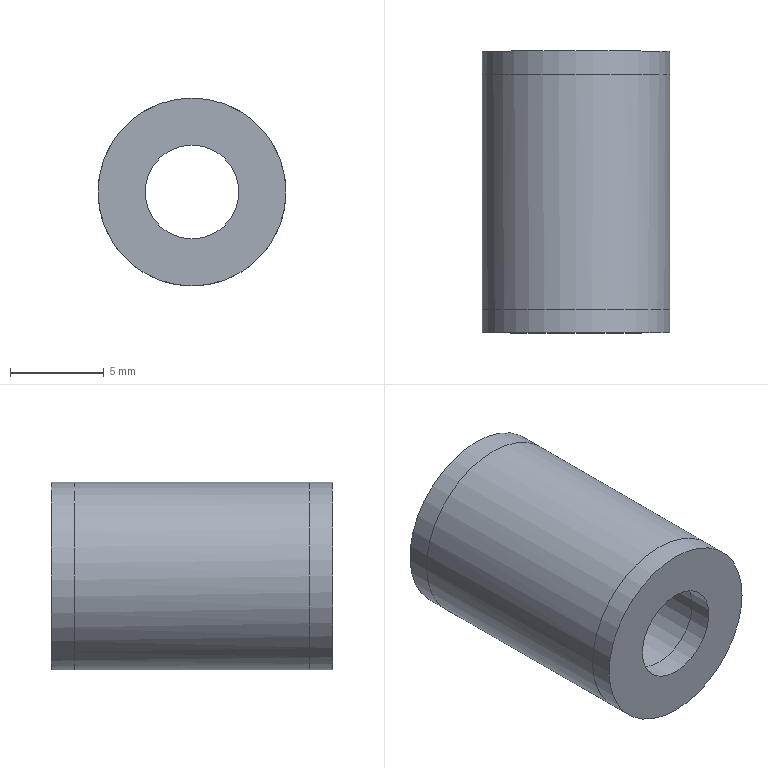Part | STEP file | solid 1 | 1 solid | 8 faces | box 10 x 15 x 10 mm | volume 148.735 mm3 | cylinder 4 | plane 4 | commonest cylinder face diameters 5 x1 5.005 x1 9.995 x1 10 x1